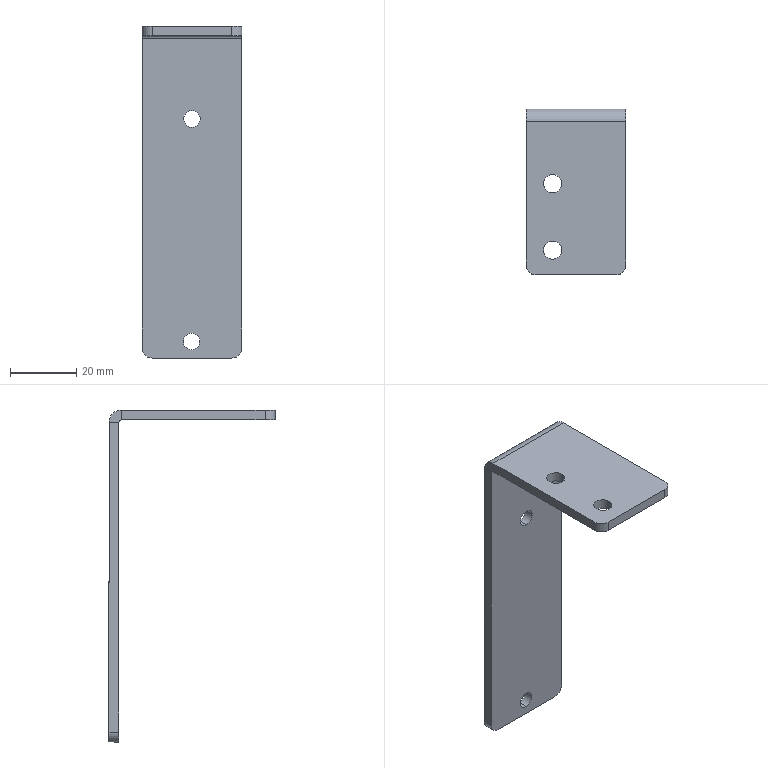Part | SolidWorks | features HoleWzd 2, EdgeFlange 1, Fillet 1, FlatPattern 1, SMBaseFlange 1, SheetMetal 1 | 1 solid | 26 faces | box 30 x 50 x 100 mm | volume 12860 mm3 | cylinder 14 | plane 12 | commonest cylinder face diameters 5 x4 5.5 x4 6 x4 1.473 x1 7.473 x1
STEP:
#1=CARTESIAN_POINT('',(-0.1445,22.,-97.5));
#2=VERTEX_POINT('',#1);
#3=CARTESIAN_POINT('',(-0.1445,22.,-92.5));
#4=VERTEX_POINT('',#3);
#5=CARTESIAN_POINT('',(-0.1445,22.,-95.));
#6=DIRECTION('',(0.,1.,0.));
#7=DIRECTION('',(0.,0.,1.));
#8=AXIS2_PLACEMENT_3D('',#5,#6,#7);
#9=CIRCLE('',#8,2.5);
#10=EDGE_CURVE('',#2,#4,#9,.T.);
#11=ORIENTED_EDGE('',*,*,#10,.F.);
#12=CARTESIAN_POINT('',(-0.1445,25.,-97.5));
#13=VERTEX_POINT('',#12);
#14=CARTESIAN_POINT('',(-0.1445,25.,-97.5));
#15=DIRECTION('',(0.,1.,0.));
#16=VECTOR('',#15,1000.);
#17=LINE('',#14,#16);
#18=EDGE_CURVE('',#2,#13,#17,.T.);
#19=ORIENTED_EDGE('',*,*,#18,.T.);
#20=CARTESIAN_POINT('',(-0.1445,25.,-92.5));
#21=VERTEX_POINT('',#20);
#22=CARTESIAN_POINT('',(-0.1445,25.,-95.));
#23=DIRECTION('',(0.,1.,0.));
#24=DIRECTION('',(0.,0.,1.));
#25=AXIS2_PLACEMENT_3D('',#22,#23,#24);
#26=CIRCLE('',#25,2.5);
#27=EDGE_CURVE('',#13,#21,#26,.T.);
#28=ORIENTED_EDGE('',*,*,#27,.T.);
#29=CARTESIAN_POINT('',(-0.1445,25.,-92.5));
#30=DIRECTION('',(0.,1.,0.));
#31=VECTOR('',#30,1000.);
#32=LINE('',#29,#31);
#33=EDGE_CURVE('',#4,#21,#32,.T.);
#34=ORIENTED_EDGE('',*,*,#33,.F.);
#35=EDGE_LOOP('',(#11,#19,#28,#34));
#36=FACE_OUTER_BOUND('',#35,.T.);
#37=CARTESIAN_POINT('',(-0.1445,25.,-95.));
#38=DIRECTION('',(0.,1.,0.));
#39=DIRECTION('',(0.,0.,1.));
#40=AXIS2_PLACEMENT_3D('',#37,#38,#39);
#41=CYLINDRICAL_SURFACE('',#40,2.5);
#42=ADVANCED_FACE('',(#36),#41,.F.);
#43=CARTESIAN_POINT('',(-0.004505,22.,-30.5));
#44=VERTEX_POINT('',#43);
#45=CARTESIAN_POINT('',(-0.004505,22.,-25.5));
#46=VERTEX_POINT('',#45);
#47=CARTESIAN_POINT('',(-0.004505,22.,-28.));
#48=DIRECTION('',(0.,1.,0.));
#49=DIRECTION('',(0.,0.,1.));
#50=AXIS2_PLACEMENT_3D('',#47,#48,#49);
#51=CIRCLE('',#50,2.5);
#52=EDGE_CURVE('',#44,#46,#51,.T.);
#53=ORIENTED_EDGE('',*,*,#52,.F.);
#54=CARTESIAN_POINT('',(-0.004505,25.,-30.5));
#55=VERTEX_POINT('',#54);
#56=CARTESIAN_POINT('',(-0.004505,25.,-30.5));
#57=DIRECTION('',(0.,1.,0.));
#58=VECTOR('',#57,1000.);
#59=LINE('',#56,#58);
#60=EDGE_CURVE('',#44,#55,#59,.T.);
#61=ORIENTED_EDGE('',*,*,#60,.T.);
#62=CARTESIAN_POINT('',(-0.004505,25.,-25.5));
#63=VERTEX_POINT('',#62);
#64=CARTESIAN_POINT('',(-0.004505,25.,-28.));
#65=DIRECTION('',(0.,1.,0.));
#66=DIRECTION('',(0.,0.,1.));
#67=AXIS2_PLACEMENT_3D('',#64,#65,#66);
#68=CIRCLE('',#67,2.5);
#69=EDGE_CURVE('',#55,#63,#68,.T.);
#70=ORIENTED_EDGE('',*,*,#69,.T.);
#71=CARTESIAN_POINT('',(-0.004505,25.,-25.5));
#72=DIRECTION('',(0.,1.,0.));
#73=VECTOR('',#72,1000.);
#74=LINE('',#71,#73);
#75=EDGE_CURVE('',#46,#63,#74,.T.);
#76=ORIENTED_EDGE('',*,*,#75,.F.);
#77=EDGE_LOOP('',(#53,#61,#70,#76));
#78=FACE_OUTER_BOUND('',#77,.T.);
#79=CARTESIAN_POINT('',(-0.004505,25.,-28.));
#80=DIRECTION('',(0.,1.,0.));
#81=DIRECTION('',(0.,0.,1.));
#82=AXIS2_PLACEMENT_3D('',#79,#80,#81);
#83=CYLINDRICAL_SURFACE('',#82,2.5);
#84=ADVANCED_FACE('',(#78),#83,.F.);
#85=CARTESIAN_POINT('',(-9.75,-17.5,-3.));
#86=VERTEX_POINT('',#85);
#87=CARTESIAN_POINT('',(-4.25,-17.5,-3.));
#88=VERTEX_POINT('',#87);
#89=CARTESIAN_POINT('',(-7.,-17.5,-3.));
#90=DIRECTION('',(0.,0.,1.));
#91=DIRECTION('',(1.,0.,0.));
#92=AXIS2_PLACEMENT_3D('',#89,#90,#91);
#93=CIRCLE('',#92,2.75);
#94=EDGE_CURVE('',#86,#88,#93,.T.);
#95=ORIENTED_EDGE('',*,*,#94,.F.);
#96=CARTESIAN_POINT('',(-9.75,-17.5,0.));
#97=VERTEX_POINT('',#96);
#98=CARTESIAN_POINT('',(-9.75,-17.5,0.));
#99=DIRECTION('',(0.,0.,1.));
#100=VECTOR('',#99,1000.);
#101=LINE('',#98,#100);
#102=EDGE_CURVE('',#86,#97,#101,.T.);
#103=ORIENTED_EDGE('',*,*,#102,.T.);
#104=CARTESIAN_POINT('',(-4.25,-17.5,0.));
#105=VERTEX_POINT('',#104);
#106=CARTESIAN_POINT('',(-7.,-17.5,0.));
#107=DIRECTION('',(0.,0.,1.));
#108=DIRECTION('',(1.,0.,0.));
#109=AXIS2_PLACEMENT_3D('',#106,#107,#108);
#110=CIRCLE('',#109,2.75);
#111=EDGE_CURVE('',#97,#105,#110,.T.);
#112=ORIENTED_EDGE('',*,*,#111,.T.);
#113=CARTESIAN_POINT('',(-4.25,-17.5,0.));
#114=DIRECTION('',(0.,0.,1.));
#115=VECTOR('',#114,1000.);
#116=LINE('',#113,#115);
#117=EDGE_CURVE('',#88,#105,#116,.T.);
#118=ORIENTED_EDGE('',*,*,#117,.F.);
#119=EDGE_LOOP('',(#95,#103,#112,#118));
#120=FACE_OUTER_BOUND('',#119,.T.);
#121=CARTESIAN_POINT('',(-7.,-17.5,0.));
#122=DIRECTION('',(0.,0.,1.));
#123=DIRECTION('',(1.,0.,0.));
#124=AXIS2_PLACEMENT_3D('',#121,#122,#123);
#125=CYLINDRICAL_SURFACE('',#124,2.75);
#126=ADVANCED_FACE('',(#120),#125,.F.);
#127=CARTESIAN_POINT('',(-9.75,2.5,-3.));
#128=VERTEX_POINT('',#127);
#129=CARTESIAN_POINT('',(-4.25,2.5,-3.));
#130=VERTEX_POINT('',#129);
#131=CARTESIAN_POINT('',(-7.,2.5,-3.));
#132=DIRECTION('',(0.,0.,1.));
#133=DIRECTION('',(1.,0.,0.));
#134=AXIS2_PLACEMENT_3D('',#131,#132,#133);
#135=CIRCLE('',#134,2.75);
#136=EDGE_CURVE('',#128,#130,#135,.T.);
#137=ORIENTED_EDGE('',*,*,#136,.F.);
#138=CARTESIAN_POINT('',(-9.75,2.5,0.));
#139=VERTEX_POINT('',#138);
#140=CARTESIAN_POINT('',(-9.75,2.5,0.));
#141=DIRECTION('',(0.,0.,1.));
#142=VECTOR('',#141,1000.);
#143=LINE('',#140,#142);
#144=EDGE_CURVE('',#128,#139,#143,.T.);
#145=ORIENTED_EDGE('',*,*,#144,.T.);
#146=CARTESIAN_POINT('',(-4.25,2.5,0.));
#147=VERTEX_POINT('',#146);
#148=CARTESIAN_POINT('',(-7.,2.5,0.));
#149=DIRECTION('',(0.,0.,1.));
#150=DIRECTION('',(1.,0.,0.));
#151=AXIS2_PLACEMENT_3D('',#148,#149,#150);
#152=CIRCLE('',#151,2.75);
#153=EDGE_CURVE('',#139,#147,#152,.T.);
#154=ORIENTED_EDGE('',*,*,#153,.T.);
#155=CARTESIAN_POINT('',(-4.25,2.5,0.));
#156=DIRECTION('',(0.,0.,1.));
#157=VECTOR('',#156,1000.);
#158=LINE('',#155,#157);
#159=EDGE_CURVE('',#130,#147,#158,.T.);
#160=ORIENTED_EDGE('',*,*,#159,.F.);
#161=EDGE_LOOP('',(#137,#145,#154,#160));
#162=FACE_OUTER_BOUND('',#161,.T.);
#163=CARTESIAN_POINT('',(-7.,2.5,0.));
#164=DIRECTION('',(0.,0.,1.));
#165=DIRECTION('',(1.,0.,0.));
#166=AXIS2_PLACEMENT_3D('',#163,#164,#165);
#167=CYLINDRICAL_SURFACE('',#166,2.75);
#168=ADVANCED_FACE('',(#162),#167,.F.);
#169=CARTESIAN_POINT('',(15.,-22.,0.));
#170=VERTEX_POINT('',#169);
#171=CARTESIAN_POINT('',(15.,21.263,0.));
#172=VERTEX_POINT('',#171);
#173=CARTESIAN_POINT('',(15.,25.,0.));
#174=DIRECTION('',(0.,1.,0.));
#175=VECTOR('',#174,1000.);
#176=LINE('',#173,#175);
#177=EDGE_CURVE('',#170,#172,#176,.T.);
#178=ORIENTED_EDGE('',*,*,#177,.F.);
#179=CARTESIAN_POINT('',(15.,-22.,-3.));
#180=VERTEX_POINT('',#179);
#181=CARTESIAN_POINT('',(15.,-22.,-3.));
#182=DIRECTION('',(0.,0.,-1.));
#183=VECTOR('',#182,1000.);
#184=LINE('',#181,#183);
#185=EDGE_CURVE('',#170,#180,#184,.T.);
#186=ORIENTED_EDGE('',*,*,#185,.T.);
#187=CARTESIAN_POINT('',(15.,21.263,-3.));
#188=VERTEX_POINT('',#187);
#189=CARTESIAN_POINT('',(15.,25.,-3.));
#190=DIRECTION('',(0.,1.,0.));
#191=VECTOR('',#190,1000.);
#192=LINE('',#189,#191);
#193=EDGE_CURVE('',#180,#188,#192,.T.);
#194=ORIENTED_EDGE('',*,*,#193,.T.);
#195=CARTESIAN_POINT('',(15.,21.263,-3.));
#196=DIRECTION('',(0.,0.,1.));
#197=VECTOR('',#196,1000.);
#198=LINE('',#195,#197);
#199=EDGE_CURVE('',#188,#172,#198,.T.);
#200=ORIENTED_EDGE('',*,*,#199,.T.);
#201=EDGE_LOOP('',(#178,#186,#194,#200));
#202=FACE_OUTER_BOUND('',#201,.T.);
#203=CARTESIAN_POINT('',(15.,25.,-3.));
#204=DIRECTION('',(1.,0.,0.));
#205=DIRECTION('',(0.,1.,0.));
#206=AXIS2_PLACEMENT_3D('',#203,#204,#205);
#207=PLANE('',#206);
#208=ADVANCED_FACE('',(#202),#207,.T.);
#209=CARTESIAN_POINT('',(-7.,-17.5,-3.));
#210=DIRECTION('',(0.,0.,1.));
#211=DIRECTION('',(1.,0.,0.));
#212=AXIS2_PLACEMENT_3D('',#209,#210,#211);
#213=CIRCLE('',#212,2.75);
#214=EDGE_CURVE('',#88,#86,#213,.T.);
#215=ORIENTED_EDGE('',*,*,#214,.T.);
#216=ORIENTED_EDGE('',*,*,#94,.T.);
#217=EDGE_LOOP('',(#215,#216));
#218=FACE_BOUND('',#217,.T.);
#219=CARTESIAN_POINT('',(-7.,2.5,-3.));
#220=DIRECTION('',(0.,0.,1.));
#221=DIRECTION('',(1.,0.,0.));
#222=AXIS2_PLACEMENT_3D('',#219,#220,#221);
#223=CIRCLE('',#222,2.75);
#224=EDGE_CURVE('',#130,#128,#223,.T.);
#225=ORIENTED_EDGE('',*,*,#224,.T.);
#226=ORIENTED_EDGE('',*,*,#136,.T.);
#227=EDGE_LOOP('',(#225,#226));
#228=FACE_BOUND('',#227,.T.);
#229=CARTESIAN_POINT('',(-12.,-25.,-3.));
#230=VERTEX_POINT('',#229);
#231=CARTESIAN_POINT('',(12.,-25.,-3.));
#232=VERTEX_POINT('',#231);
#233=CARTESIAN_POINT('',(-15.,-25.,-3.));
#234=DIRECTION('',(1.,0.,0.));
#235=VECTOR('',#234,1000.);
#236=LINE('',#233,#235);
#237=EDGE_CURVE('',#230,#232,#236,.T.);
#238=ORIENTED_EDGE('',*,*,#237,.F.);
#239=CARTESIAN_POINT('',(-15.,-22.,-3.));
#240=VERTEX_POINT('',#239);
#241=CARTESIAN_POINT('',(-12.,-22.,-3.));
#242=DIRECTION('',(0.,0.,-1.));
#243=DIRECTION('',(1.,0.,0.));
#244=AXIS2_PLACEMENT_3D('',#241,#242,#243);
#245=CIRCLE('',#244,3.);
#246=EDGE_CURVE('',#230,#240,#245,.T.);
#247=ORIENTED_EDGE('',*,*,#246,.T.);
#248=CARTESIAN_POINT('',(-15.,21.263,-3.));
#249=VERTEX_POINT('',#248);
#250=CARTESIAN_POINT('',(-15.,25.,-3.));
#251=DIRECTION('',(0.,-1.,0.));
#252=VECTOR('',#251,1000.);
#253=LINE('',#250,#252);
#254=EDGE_CURVE('',#249,#240,#253,.T.);
#255=ORIENTED_EDGE('',*,*,#254,.F.);
#256=CARTESIAN_POINT('',(15.,21.263,-3.));
#257=DIRECTION('',(-1.,0.,0.));
#258=VECTOR('',#257,1000.);
#259=LINE('',#256,#258);
#260=EDGE_CURVE('',#188,#249,#259,.T.);
#261=ORIENTED_EDGE('',*,*,#260,.F.);
#262=ORIENTED_EDGE('',*,*,#193,.F.);
#263=CARTESIAN_POINT('',(12.,-22.,-3.));
#264=DIRECTION('',(0.,0.,-1.));
#265=DIRECTION('',(1.,0.,0.));
#266=AXIS2_PLACEMENT_3D('',#263,#264,#265);
#267=CIRCLE('',#266,3.);
#268=EDGE_CURVE('',#180,#232,#267,.T.);
#269=ORIENTED_EDGE('',*,*,#268,.T.);
#270=EDGE_LOOP('',(#238,#247,#255,#261,#262,#269));
#271=FACE_OUTER_BOUND('',#270,.T.);
#272=CARTESIAN_POINT('',(0.,0.,-3.));
#273=DIRECTION('',(0.,0.,1.));
#274=DIRECTION('',(1.,0.,0.));
#275=AXIS2_PLACEMENT_3D('',#272,#273,#274);
#276=PLANE('',#275);
#277=ADVANCED_FACE('',(#218,#228,#271),#276,.F.);
#278=CARTESIAN_POINT('',(-7.,-17.5,0.));
#279=DIRECTION('',(0.,0.,1.));
#280=DIRECTION('',(1.,0.,0.));
#281=AXIS2_PLACEMENT_3D('',#278,#279,#280);
#282=CIRCLE('',#281,2.75);
#283=EDGE_CURVE('',#105,#97,#282,.T.);
#284=ORIENTED_EDGE('',*,*,#283,.F.);
#285=ORIENTED_EDGE('',*,*,#111,.F.);
#286=EDGE_LOOP('',(#284,#285));
#287=FACE_BOUND('',#286,.T.);
#288=CARTESIAN_POINT('',(-7.,2.5,0.));
#289=DIRECTION('',(0.,0.,1.));
#290=DIRECTION('',(1.,0.,0.));
#291=AXIS2_PLACEMENT_3D('',#288,#289,#290);
#292=CIRCLE('',#291,2.75);
#293=EDGE_CURVE('',#147,#139,#292,.T.);
#294=ORIENTED_EDGE('',*,*,#293,.F.);
#295=ORIENTED_EDGE('',*,*,#153,.F.);
#296=EDGE_LOOP('',(#294,#295));
#297=FACE_BOUND('',#296,.T.);
#298=CARTESIAN_POINT('',(-15.,21.263,0.));
#299=VERTEX_POINT('',#298);
#300=CARTESIAN_POINT('',(-15.,-22.,0.));
#301=VERTEX_POINT('',#300);
#302=CARTESIAN_POINT('',(-15.,25.,0.));
#303=DIRECTION('',(0.,-1.,0.));
#304=VECTOR('',#303,1000.);
#305=LINE('',#302,#304);
#306=EDGE_CURVE('',#299,#301,#305,.T.);
#307=ORIENTED_EDGE('',*,*,#306,.T.);
#308=CARTESIAN_POINT('',(-12.,-25.,0.));
#309=VERTEX_POINT('',#308);
#310=CARTESIAN_POINT('',(-12.,-22.,0.));
#311=DIRECTION('',(0.,0.,1.));
#312=DIRECTION('',(1.,0.,0.));
#313=AXIS2_PLACEMENT_3D('',#310,#311,#312);
#314=CIRCLE('',#313,3.);
#315=EDGE_CURVE('',#301,#309,#314,.T.);
#316=ORIENTED_EDGE('',*,*,#315,.T.);
#317=CARTESIAN_POINT('',(12.,-25.,0.));
#318=VERTEX_POINT('',#317);
#319=CARTESIAN_POINT('',(-15.,-25.,0.));
#320=DIRECTION('',(1.,0.,0.));
#321=VECTOR('',#320,1000.);
#322=LINE('',#319,#321);
#323=EDGE_CURVE('',#309,#318,#322,.T.);
#324=ORIENTED_EDGE('',*,*,#323,.T.);
#325=CARTESIAN_POINT('',(12.,-22.,0.));
#326=DIRECTION('',(0.,0.,1.));
#327=DIRECTION('',(1.,0.,0.));
#328=AXIS2_PLACEMENT_3D('',#325,#326,#327);
#329=CIRCLE('',#328,3.);
#330=EDGE_CURVE('',#318,#170,#329,.T.);
#331=ORIENTED_EDGE('',*,*,#330,.T.);
#332=ORIENTED_EDGE('',*,*,#177,.T.);
#333=CARTESIAN_POINT('',(15.,21.263,0.));
#334=DIRECTION('',(-1.,0.,0.));
#335=VECTOR('',#334,1000.);
#336=LINE('',#333,#335);
#337=EDGE_CURVE('',#172,#299,#336,.T.);
#338=ORIENTED_EDGE('',*,*,#337,.T.);
#339=EDGE_LOOP('',(#307,#316,#324,#331,#332,#338));
#340=FACE_OUTER_BOUND('',#339,.T.);
#341=CARTESIAN_POINT('',(0.,0.,0.));
#342=DIRECTION('',(0.,0.,1.));
#343=DIRECTION('',(1.,0.,0.));
#344=AXIS2_PLACEMENT_3D('',#341,#342,#343);
#345=PLANE('',#344);
#346=ADVANCED_FACE('',(#287,#297,#340),#345,.T.);
#347=ORIENTED_EDGE('',*,*,#323,.F.);
#348=CARTESIAN_POINT('',(-12.,-25.,-3.));
#349=DIRECTION('',(0.,0.,-1.));
#350=VECTOR('',#349,1000.);
#351=LINE('',#348,#350);
#352=EDGE_CURVE('',#309,#230,#351,.T.);
#353=ORIENTED_EDGE('',*,*,#352,.T.);
#354=ORIENTED_EDGE('',*,*,#237,.T.);
#355=CARTESIAN_POINT('',(12.,-25.,-3.));
#356=DIRECTION('',(0.,0.,1.));
#357=VECTOR('',#356,1000.);
#358=LINE('',#355,#357);
#359=EDGE_CURVE('',#232,#318,#358,.T.);
#360=ORIENTED_EDGE('',*,*,#359,.T.);
#361=EDGE_LOOP('',(#347,#353,#354,#360));
#362=FACE_OUTER_BOUND('',#361,.T.);
#363=CARTESIAN_POINT('',(-15.,-25.,-3.));
#364=DIRECTION('',(0.,-1.,0.));
#365=DIRECTION('',(0.,0.,-1.));
#366=AXIS2_PLACEMENT_3D('',#363,#364,#365);
#367=PLANE('',#366);
#368=ADVANCED_FACE('',(#362),#367,.T.);
#369=ORIENTED_EDGE('',*,*,#254,.T.);
#370=CARTESIAN_POINT('',(-15.,-22.,-3.));
#371=DIRECTION('',(0.,0.,1.));
#372=VECTOR('',#371,1000.);
#373=LINE('',#370,#372);
#374=EDGE_CURVE('',#240,#301,#373,.T.);
#375=ORIENTED_EDGE('',*,*,#374,.T.);
#376=ORIENTED_EDGE('',*,*,#306,.F.);
#377=CARTESIAN_POINT('',(-15.,21.263,-3.));
#378=DIRECTION('',(0.,0.,1.));
#379=VECTOR('',#378,1000.);
#380=LINE('',#377,#379);
#381=EDGE_CURVE('',#249,#299,#380,.T.);
#382=ORIENTED_EDGE('',*,*,#381,.F.);
#383=EDGE_LOOP('',(#369,#375,#376,#382));
#384=FACE_OUTER_BOUND('',#383,.T.);
#385=CARTESIAN_POINT('',(-15.,25.,-3.));
#386=DIRECTION('',(-1.,0.,0.));
#387=DIRECTION('',(0.,-1.,0.));
#388=AXIS2_PLACEMENT_3D('',#385,#386,#387);
#389=PLANE('',#388);
#390=ADVANCED_FACE('',(#384),#389,.T.);
#391=CARTESIAN_POINT('',(-15.,22.,-3.737));
#392=VERTEX_POINT('',#391);
#393=CARTESIAN_POINT('',(-15.,25.,-3.737));
#394=VERTEX_POINT('',#393);
#395=CARTESIAN_POINT('',(-15.,25.,-3.737));
#396=DIRECTION('',(0.,1.,0.));
#397=VECTOR('',#396,1000.);
#398=LINE('',#395,#397);
#399=EDGE_CURVE('',#392,#394,#398,.T.);
#400=ORIENTED_EDGE('',*,*,#399,.F.);
#401=CARTESIAN_POINT('',(-15.,21.263,-3.737));
#402=DIRECTION('',(-1.,0.,0.));
#403=DIRECTION('',(0.,0.,-1.));
#404=AXIS2_PLACEMENT_3D('',#401,#402,#403);
#405=CIRCLE('',#404,0.7366);
#406=EDGE_CURVE('',#249,#392,#405,.T.);
#407=ORIENTED_EDGE('',*,*,#406,.F.);
#408=ORIENTED_EDGE('',*,*,#381,.T.);
#409=CARTESIAN_POINT('',(-15.,21.263,-3.737));
#410=DIRECTION('',(-1.,0.,0.));
#411=DIRECTION('',(0.,0.,-1.));
#412=AXIS2_PLACEMENT_3D('',#409,#410,#411);
#413=CIRCLE('',#412,3.737);
#414=EDGE_CURVE('',#299,#394,#413,.T.);
#415=ORIENTED_EDGE('',*,*,#414,.T.);
#416=EDGE_LOOP('',(#400,#407,#408,#415));
#417=FACE_OUTER_BOUND('',#416,.T.);
#418=CARTESIAN_POINT('',(-15.,21.263,-3.737));
#419=DIRECTION('',(-1.,0.,0.));
#420=DIRECTION('',(0.,0.,1.));
#421=AXIS2_PLACEMENT_3D('',#418,#419,#420);
#422=PLANE('',#421);
#423=ADVANCED_FACE('',(#417),#422,.T.);
#424=CARTESIAN_POINT('',(15.,22.,-3.737));
#425=VERTEX_POINT('',#424);
#426=CARTESIAN_POINT('',(15.,21.263,-3.737));
#427=DIRECTION('',(1.,0.,0.));
#428=DIRECTION('',(0.,0.,-1.));
#429=AXIS2_PLACEMENT_3D('',#426,#427,#428);
#430=CIRCLE('',#429,0.7366);
#431=EDGE_CURVE('',#425,#188,#430,.T.);
#432=ORIENTED_EDGE('',*,*,#431,.F.);
#433=CARTESIAN_POINT('',(15.,25.,-3.737));
#434=VERTEX_POINT('',#433);
#435=CARTESIAN_POINT('',(15.,22.,-3.737));
#436=DIRECTION('',(0.,1.,0.));
#437=VECTOR('',#436,1000.);
#438=LINE('',#435,#437);
#439=EDGE_CURVE('',#425,#434,#438,.T.);
#440=ORIENTED_EDGE('',*,*,#439,.T.);
#441=CARTESIAN_POINT('',(15.,21.263,-3.737));
#442=DIRECTION('',(1.,0.,0.));
#443=DIRECTION('',(0.,0.,-1.));
#444=AXIS2_PLACEMENT_3D('',#441,#442,#443);
#445=CIRCLE('',#444,3.737);
#446=EDGE_CURVE('',#434,#172,#445,.T.);
#447=ORIENTED_EDGE('',*,*,#446,.T.);
#448=ORIENTED_EDGE('',*,*,#199,.F.);
#449=EDGE_LOOP('',(#432,#440,#447,#448));
#450=FACE_OUTER_BOUND('',#449,.T.);
#451=CARTESIAN_POINT('',(15.,21.263,-3.737));
#452=DIRECTION('',(-1.,0.,0.));
#453=DIRECTION('',(0.,0.,1.));
#454=AXIS2_PLACEMENT_3D('',#451,#452,#453);
#455=PLANE('',#454);
#456=ADVANCED_FACE('',(#450),#455,.F.);
#457=ORIENTED_EDGE('',*,*,#337,.F.);
#458=ORIENTED_EDGE('',*,*,#446,.F.);
#459=CARTESIAN_POINT('',(0.,25.,-3.737));
#460=DIRECTION('',(1.,0.,0.));
#461=VECTOR('',#460,1000.);
#462=LINE('',#459,#461);
#463=EDGE_CURVE('',#394,#434,#462,.T.);
#464=ORIENTED_EDGE('',*,*,#463,.F.);
#465=ORIENTED_EDGE('',*,*,#414,.F.);
#466=EDGE_LOOP('',(#457,#458,#464,#465));
#467=FACE_OUTER_BOUND('',#466,.T.);
#468=CARTESIAN_POINT('',(15.,21.263,-3.737));
#469=DIRECTION('',(1.,0.,0.));
#470=DIRECTION('',(0.,1.,0.));
#471=AXIS2_PLACEMENT_3D('',#468,#469,#470);
#472=CYLINDRICAL_SURFACE('',#471,3.737);
#473=ADVANCED_FACE('',(#467),#472,.T.);
#474=ORIENTED_EDGE('',*,*,#260,.T.);
#475=ORIENTED_EDGE('',*,*,#406,.T.);
#476=CARTESIAN_POINT('',(-15.,22.,-3.737));
#477=DIRECTION('',(1.,0.,0.));
#478=VECTOR('',#477,1000.);
#479=LINE('',#476,#478);
#480=EDGE_CURVE('',#392,#425,#479,.T.);
#481=ORIENTED_EDGE('',*,*,#480,.T.);
#482=ORIENTED_EDGE('',*,*,#431,.T.);
#483=EDGE_LOOP('',(#474,#475,#481,#482));
#484=FACE_OUTER_BOUND('',#483,.T.);
#485=CARTESIAN_POINT('',(15.,21.263,-3.737));
#486=DIRECTION('',(1.,0.,0.));
#487=DIRECTION('',(0.,1.,0.));
#488=AXIS2_PLACEMENT_3D('',#485,#486,#487);
#489=CYLINDRICAL_SURFACE('',#488,0.7366);
#490=ADVANCED_FACE('',(#484),#489,.F.);
#491=CARTESIAN_POINT('',(15.,22.,-97.));
#492=VERTEX_POINT('',#491);
#493=CARTESIAN_POINT('',(15.,22.,0.));
#494=DIRECTION('',(0.,0.,1.));
#495=VECTOR('',#494,1000.);
#496=LINE('',#493,#495);
#497=EDGE_CURVE('',#492,#425,#496,.T.);
#498=ORIENTED_EDGE('',*,*,#497,.F.);
#499=CARTESIAN_POINT('',(15.,25.,-97.));
#500=VERTEX_POINT('',#499);
#501=CARTESIAN_POINT('',(15.,25.,-97.));
#502=DIRECTION('',(0.,1.,0.));
#503=VECTOR('',#502,1000.);
#504=LINE('',#501,#503);
#505=EDGE_CURVE('',#492,#500,#504,.T.);
#506=ORIENTED_EDGE('',*,*,#505,.T.);
#507=CARTESIAN_POINT('',(15.,25.,-3.));
#508=DIRECTION('',(0.,0.,1.));
#509=VECTOR('',#508,1000.);
#510=LINE('',#507,#509);
#511=EDGE_CURVE('',#500,#434,#510,.T.);
#512=ORIENTED_EDGE('',*,*,#511,.T.);
#513=ORIENTED_EDGE('',*,*,#439,.F.);
#514=EDGE_LOOP('',(#498,#506,#512,#513));
#515=FACE_OUTER_BOUND('',#514,.T.);
#516=CARTESIAN_POINT('',(15.,25.,-3.));
#517=DIRECTION('',(1.,0.,0.));
#518=DIRECTION('',(0.,0.,-1.));
#519=AXIS2_PLACEMENT_3D('',#516,#517,#518);
#520=PLANE('',#519);
#521=ADVANCED_FACE('',(#515),#520,.T.);
#522=CARTESIAN_POINT('',(-15.,25.,-97.));
#523=VERTEX_POINT('',#522);
#524=CARTESIAN_POINT('',(-15.,25.,-100.));
#525=DIRECTION('',(0.,0.,-1.));
#526=VECTOR('',#525,1000.);
#527=LINE('',#524,#526);
#528=EDGE_CURVE('',#394,#523,#527,.T.);
#529=ORIENTED_EDGE('',*,*,#528,.T.);
#530=CARTESIAN_POINT('',(-15.,22.,-97.));
#531=VERTEX_POINT('',#530);
#532=CARTESIAN_POINT('',(-15.,25.,-97.));
#533=DIRECTION('',(0.,-1.,0.));
#534=VECTOR('',#533,1000.);
#535=LINE('',#532,#534);
#536=EDGE_CURVE('',#523,#531,#535,.T.);
#537=ORIENTED_EDGE('',*,*,#536,.T.);
#538=CARTESIAN_POINT('',(-15.,22.,0.));
#539=DIRECTION('',(0.,0.,-1.));
#540=VECTOR('',#539,1000.);
#541=LINE('',#538,#540);
#542=EDGE_CURVE('',#392,#531,#541,.T.);
#543=ORIENTED_EDGE('',*,*,#542,.F.);
#544=ORIENTED_EDGE('',*,*,#399,.T.);
#545=EDGE_LOOP('',(#529,#537,#543,#544));
#546=FACE_OUTER_BOUND('',#545,.T.);
#547=CARTESIAN_POINT('',(-15.,25.,-100.));
#548=DIRECTION('',(-1.,0.,0.));
#549=DIRECTION('',(0.,0.,1.));
#550=AXIS2_PLACEMENT_3D('',#547,#548,#549);
#551=PLANE('',#550);
#552=ADVANCED_FACE('',(#546),#551,.T.);
#553=CARTESIAN_POINT('',(-0.1445,25.,-95.));
#554=DIRECTION('',(0.,1.,0.));
#555=DIRECTION('',(0.,0.,1.));
#556=AXIS2_PLACEMENT_3D('',#553,#554,#555);
#557=CIRCLE('',#556,2.5);
#558=EDGE_CURVE('',#21,#13,#557,.T.);
#559=ORIENTED_EDGE('',*,*,#558,.F.);
#560=ORIENTED_EDGE('',*,*,#27,.F.);
#561=EDGE_LOOP('',(#559,#560));
#562=FACE_BOUND('',#561,.T.);
#563=CARTESIAN_POINT('',(-0.004505,25.,-28.));
#564=DIRECTION('',(0.,1.,0.));
#565=DIRECTION('',(0.,0.,1.));
#566=AXIS2_PLACEMENT_3D('',#563,#564,#565);
#567=CIRCLE('',#566,2.5);
#568=EDGE_CURVE('',#63,#55,#567,.T.);
#569=ORIENTED_EDGE('',*,*,#568,.F.);
#570=ORIENTED_EDGE('',*,*,#69,.F.);
#571=EDGE_LOOP('',(#569,#570));
#572=FACE_BOUND('',#571,.T.);
#573=CARTESIAN_POINT('',(-12.,25.,-100.));
#574=VERTEX_POINT('',#573);
#575=CARTESIAN_POINT('',(12.,25.,-100.));
#576=VERTEX_POINT('',#575);
#577=CARTESIAN_POINT('',(15.,25.,-100.));
#578=DIRECTION('',(1.,0.,0.));
#579=VECTOR('',#578,1000.);
#580=LINE('',#577,#579);
#581=EDGE_CURVE('',#574,#576,#580,.T.);
#582=ORIENTED_EDGE('',*,*,#581,.F.);
#583=CARTESIAN_POINT('',(-12.,25.,-97.));
#584=DIRECTION('',(0.,1.,0.));
#585=DIRECTION('',(0.,0.,1.));
#586=AXIS2_PLACEMENT_3D('',#583,#584,#585);
#587=CIRCLE('',#586,3.);
#588=EDGE_CURVE('',#574,#523,#587,.T.);
#589=ORIENTED_EDGE('',*,*,#588,.T.);
#590=ORIENTED_EDGE('',*,*,#528,.F.);
#591=ORIENTED_EDGE('',*,*,#463,.T.);
#592=ORIENTED_EDGE('',*,*,#511,.F.);
#593=CARTESIAN_POINT('',(12.,25.,-97.));
#594=DIRECTION('',(0.,1.,0.));
#595=DIRECTION('',(0.,0.,1.));
#596=AXIS2_PLACEMENT_3D('',#593,#594,#595);
#597=CIRCLE('',#596,3.);
#598=EDGE_CURVE('',#500,#576,#597,.T.);
#599=ORIENTED_EDGE('',*,*,#598,.T.);
#600=EDGE_LOOP('',(#582,#589,#590,#591,#592,#599));
#601=FACE_OUTER_BOUND('',#600,.T.);
#602=CARTESIAN_POINT('',(0.,25.,0.));
#603=DIRECTION('',(0.,1.,0.));
#604=DIRECTION('',(0.,0.,1.));
#605=AXIS2_PLACEMENT_3D('',#602,#603,#604);
#606=PLANE('',#605);
#607=ADVANCED_FACE('',(#562,#572,#601),#606,.T.);
#608=CARTESIAN_POINT('',(-0.1445,22.,-95.));
#609=DIRECTION('',(0.,1.,0.));
#610=DIRECTION('',(0.,0.,1.));
#611=AXIS2_PLACEMENT_3D('',#608,#609,#610);
#612=CIRCLE('',#611,2.5);
#613=EDGE_CURVE('',#4,#2,#612,.T.);
#614=ORIENTED_EDGE('',*,*,#613,.T.);
#615=ORIENTED_EDGE('',*,*,#10,.T.);
#616=EDGE_LOOP('',(#614,#615));
#617=FACE_BOUND('',#616,.T.);
#618=CARTESIAN_POINT('',(-0.004505,22.,-28.));
#619=DIRECTION('',(0.,1.,0.));
#620=DIRECTION('',(0.,0.,1.));
#621=AXIS2_PLACEMENT_3D('',#618,#619,#620);
#622=CIRCLE('',#621,2.5);
#623=EDGE_CURVE('',#46,#44,#622,.T.);
#624=ORIENTED_EDGE('',*,*,#623,.T.);
#625=ORIENTED_EDGE('',*,*,#52,.T.);
#626=EDGE_LOOP('',(#624,#625));
#627=FACE_BOUND('',#626,.T.);
#628=ORIENTED_EDGE('',*,*,#542,.T.);
#629=CARTESIAN_POINT('',(-12.,22.,-100.));
#630=VERTEX_POINT('',#629);
#631=CARTESIAN_POINT('',(-12.,22.,-97.));
#632=DIRECTION('',(0.,-1.,0.));
#633=DIRECTION('',(0.,0.,1.));
#634=AXIS2_PLACEMENT_3D('',#631,#632,#633);
#635=CIRCLE('',#634,3.);
#636=EDGE_CURVE('',#531,#630,#635,.T.);
#637=ORIENTED_EDGE('',*,*,#636,.T.);
#638=CARTESIAN_POINT('',(12.,22.,-100.));
#639=VERTEX_POINT('',#638);
#640=CARTESIAN_POINT('',(0.,22.,-100.));
#641=DIRECTION('',(1.,0.,0.));
#642=VECTOR('',#641,1000.);
#643=LINE('',#640,#642);
#644=EDGE_CURVE('',#630,#639,#643,.T.);
#645=ORIENTED_EDGE('',*,*,#644,.T.);
#646=CARTESIAN_POINT('',(12.,22.,-97.));
#647=DIRECTION('',(0.,-1.,0.));
#648=DIRECTION('',(0.,0.,1.));
#649=AXIS2_PLACEMENT_3D('',#646,#647,#648);
#650=CIRCLE('',#649,3.);
#651=EDGE_CURVE('',#639,#492,#650,.T.);
#652=ORIENTED_EDGE('',*,*,#651,.T.);
#653=ORIENTED_EDGE('',*,*,#497,.T.);
#654=ORIENTED_EDGE('',*,*,#480,.F.);
#655=EDGE_LOOP('',(#628,#637,#645,#652,#653,#654));
#656=FACE_OUTER_BOUND('',#655,.T.);
#657=CARTESIAN_POINT('',(0.,22.,0.));
#658=DIRECTION('',(0.,1.,0.));
#659=DIRECTION('',(0.,0.,1.));
#660=AXIS2_PLACEMENT_3D('',#657,#658,#659);
#661=PLANE('',#660);
#662=ADVANCED_FACE('',(#617,#627,#656),#661,.F.);
#663=ORIENTED_EDGE('',*,*,#644,.F.);
#664=CARTESIAN_POINT('',(-12.,25.,-100.));
#665=DIRECTION('',(0.,1.,0.));
#666=VECTOR('',#665,1000.);
#667=LINE('',#664,#666);
#668=EDGE_CURVE('',#630,#574,#667,.T.);
#669=ORIENTED_EDGE('',*,*,#668,.T.);
#670=ORIENTED_EDGE('',*,*,#581,.T.);
#671=CARTESIAN_POINT('',(12.,25.,-100.));
#672=DIRECTION('',(0.,-1.,0.));
#673=VECTOR('',#672,1000.);
#674=LINE('',#671,#673);
#675=EDGE_CURVE('',#576,#639,#674,.T.);
#676=ORIENTED_EDGE('',*,*,#675,.T.);
#677=EDGE_LOOP('',(#663,#669,#670,#676));
#678=FACE_OUTER_BOUND('',#677,.T.);
#679=CARTESIAN_POINT('',(15.,25.,-100.));
#680=DIRECTION('',(0.,0.,-1.));
#681=DIRECTION('',(0.,1.,0.));
#682=AXIS2_PLACEMENT_3D('',#679,#680,#681);
#683=PLANE('',#682);
#684=ADVANCED_FACE('',(#678),#683,.T.);
#685=ORIENTED_EDGE('',*,*,#144,.F.);
#686=ORIENTED_EDGE('',*,*,#224,.F.);
#687=ORIENTED_EDGE('',*,*,#159,.T.);
#688=ORIENTED_EDGE('',*,*,#293,.T.);
#689=EDGE_LOOP('',(#685,#686,#687,#688));
#690=FACE_OUTER_BOUND('',#689,.T.);
#691=CARTESIAN_POINT('',(-7.,2.5,0.));
#692=DIRECTION('',(0.,0.,1.));
#693=DIRECTION('',(1.,0.,0.));
#694=AXIS2_PLACEMENT_3D('',#691,#692,#693);
#695=CYLINDRICAL_SURFACE('',#694,2.75);
#696=ADVANCED_FACE('',(#690),#695,.F.);
#697=ORIENTED_EDGE('',*,*,#102,.F.);
#698=ORIENTED_EDGE('',*,*,#214,.F.);
#699=ORIENTED_EDGE('',*,*,#117,.T.);
#700=ORIENTED_EDGE('',*,*,#283,.T.);
#701=EDGE_LOOP('',(#697,#698,#699,#700));
#702=FACE_OUTER_BOUND('',#701,.T.);
#703=CARTESIAN_POINT('',(-7.,-17.5,0.));
#704=DIRECTION('',(0.,0.,1.));
#705=DIRECTION('',(1.,0.,0.));
#706=AXIS2_PLACEMENT_3D('',#703,#704,#705);
#707=CYLINDRICAL_SURFACE('',#706,2.75);
#708=ADVANCED_FACE('',(#702),#707,.F.);
#709=ORIENTED_EDGE('',*,*,#246,.F.);
#710=ORIENTED_EDGE('',*,*,#352,.F.);
#711=ORIENTED_EDGE('',*,*,#315,.F.);
#712=ORIENTED_EDGE('',*,*,#374,.F.);
#713=EDGE_LOOP('',(#709,#710,#711,#712));
#714=FACE_OUTER_BOUND('',#713,.T.);
#715=CARTESIAN_POINT('',(-12.,-22.,-3.));
#716=DIRECTION('',(0.,0.,1.));
#717=DIRECTION('',(1.,0.,0.));
#718=AXIS2_PLACEMENT_3D('',#715,#716,#717);
#719=CYLINDRICAL_SURFACE('',#718,3.);
#720=ADVANCED_FACE('',(#714),#719,.T.);
#721=ORIENTED_EDGE('',*,*,#268,.F.);
#722=ORIENTED_EDGE('',*,*,#185,.F.);
#723=ORIENTED_EDGE('',*,*,#330,.F.);
#724=ORIENTED_EDGE('',*,*,#359,.F.);
#725=EDGE_LOOP('',(#721,#722,#723,#724));
#726=FACE_OUTER_BOUND('',#725,.T.);
#727=CARTESIAN_POINT('',(12.,-22.,-3.));
#728=DIRECTION('',(0.,0.,1.));
#729=DIRECTION('',(1.,0.,0.));
#730=AXIS2_PLACEMENT_3D('',#727,#728,#729);
#731=CYLINDRICAL_SURFACE('',#730,3.);
#732=ADVANCED_FACE('',(#726),#731,.T.);
#733=ORIENTED_EDGE('',*,*,#588,.F.);
#734=ORIENTED_EDGE('',*,*,#668,.F.);
#735=ORIENTED_EDGE('',*,*,#636,.F.);
#736=ORIENTED_EDGE('',*,*,#536,.F.);
#737=EDGE_LOOP('',(#733,#734,#735,#736));
#738=FACE_OUTER_BOUND('',#737,.T.);
#739=CARTESIAN_POINT('',(-12.,25.,-97.));
#740=DIRECTION('',(0.,-1.,0.));
#741=DIRECTION('',(0.,0.,-1.));
#742=AXIS2_PLACEMENT_3D('',#739,#740,#741);
#743=CYLINDRICAL_SURFACE('',#742,3.);
#744=ADVANCED_FACE('',(#738),#743,.T.);
#745=ORIENTED_EDGE('',*,*,#598,.F.);
#746=ORIENTED_EDGE('',*,*,#505,.F.);
#747=ORIENTED_EDGE('',*,*,#651,.F.);
#748=ORIENTED_EDGE('',*,*,#675,.F.);
#749=EDGE_LOOP('',(#745,#746,#747,#748));
#750=FACE_OUTER_BOUND('',#749,.T.);
#751=CARTESIAN_POINT('',(12.,25.,-97.));
#752=DIRECTION('',(0.,-1.,0.));
#753=DIRECTION('',(0.,0.,-1.));
#754=AXIS2_PLACEMENT_3D('',#751,#752,#753);
#755=CYLINDRICAL_SURFACE('',#754,3.);
#756=ADVANCED_FACE('',(#750),#755,.T.);
#757=ORIENTED_EDGE('',*,*,#60,.F.);
#758=ORIENTED_EDGE('',*,*,#623,.F.);
#759=ORIENTED_EDGE('',*,*,#75,.T.);
#760=ORIENTED_EDGE('',*,*,#568,.T.);
#761=EDGE_LOOP('',(#757,#758,#759,#760));
#762=FACE_OUTER_BOUND('',#761,.T.);
#763=CARTESIAN_POINT('',(-0.004505,25.,-28.));
#764=DIRECTION('',(0.,1.,0.));
#765=DIRECTION('',(0.,0.,1.));
#766=AXIS2_PLACEMENT_3D('',#763,#764,#765);
#767=CYLINDRICAL_SURFACE('',#766,2.5);
#768=ADVANCED_FACE('',(#762),#767,.F.);
#769=ORIENTED_EDGE('',*,*,#18,.F.);
#770=ORIENTED_EDGE('',*,*,#613,.F.);
#771=ORIENTED_EDGE('',*,*,#33,.T.);
#772=ORIENTED_EDGE('',*,*,#558,.T.);
#773=EDGE_LOOP('',(#769,#770,#771,#772));
#774=FACE_OUTER_BOUND('',#773,.T.);
#775=CARTESIAN_POINT('',(-0.1445,25.,-95.));
#776=DIRECTION('',(0.,1.,0.));
#777=DIRECTION('',(0.,0.,1.));
#778=AXIS2_PLACEMENT_3D('',#775,#776,#777);
#779=CYLINDRICAL_SURFACE('',#778,2.5);
#780=ADVANCED_FACE('',(#774),#779,.F.);
#781=CLOSED_SHELL('',(#42,#84,#126,#168,#208,#277,#346,#368,#390,#423,#456,#473,#490,#521,#552,#607,#662,#684,#696,#708,#720,#732,#744,#756,#768,#780));
#782=MANIFOLD_SOLID_BREP('',#781);
#783=CARTESIAN_POINT('',(0.,0.,0.));
#784=DIRECTION('',(0.,0.,1.));
#785=DIRECTION('',(1.,0.,0.));
#786=AXIS2_PLACEMENT_3D('',#783,#784,#785);
#787=(LENGTH_UNIT()NAMED_UNIT(*)SI_UNIT(.MILLI.,.METRE.));
#788=UNCERTAINTY_MEASURE_WITH_UNIT(LENGTH_MEASURE(0.00001),#787,'','');
#789=(NAMED_UNIT(*)PLANE_ANGLE_UNIT()SI_UNIT($,.RADIAN.));
#790=(NAMED_UNIT(*)SI_UNIT($,.STERADIAN.)SOLID_ANGLE_UNIT());
#791=(GEOMETRIC_REPRESENTATION_CONTEXT(3)GLOBAL_UNCERTAINTY_ASSIGNED_CONTEXT((#788))GLOBAL_UNIT_ASSIGNED_CONTEXT((#787,#789,#790))REPRESENTATION_CONTEXT('',''));
#792=ADVANCED_BREP_SHAPE_REPRESENTATION('',(#782,#786),#791);